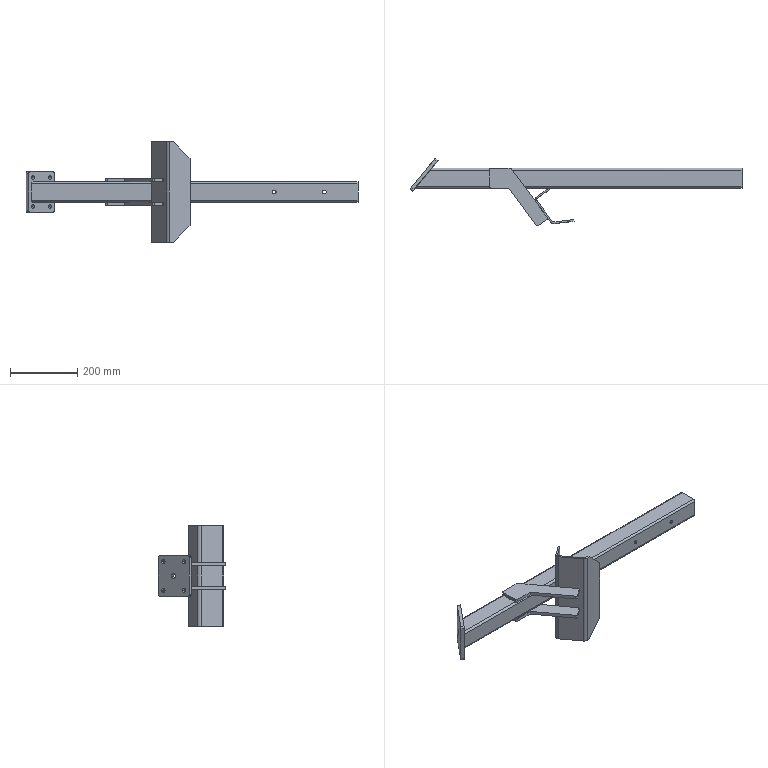Part | 5 solids | 97 faces | box 990.536 x 201.99 x 300 mm | volume 1255097 mm3 | plane 52 | cylinder 45 | commonest cylinder face diameters 10 x15 11 x8 13 x8 6 x4 12 x4 20 x4